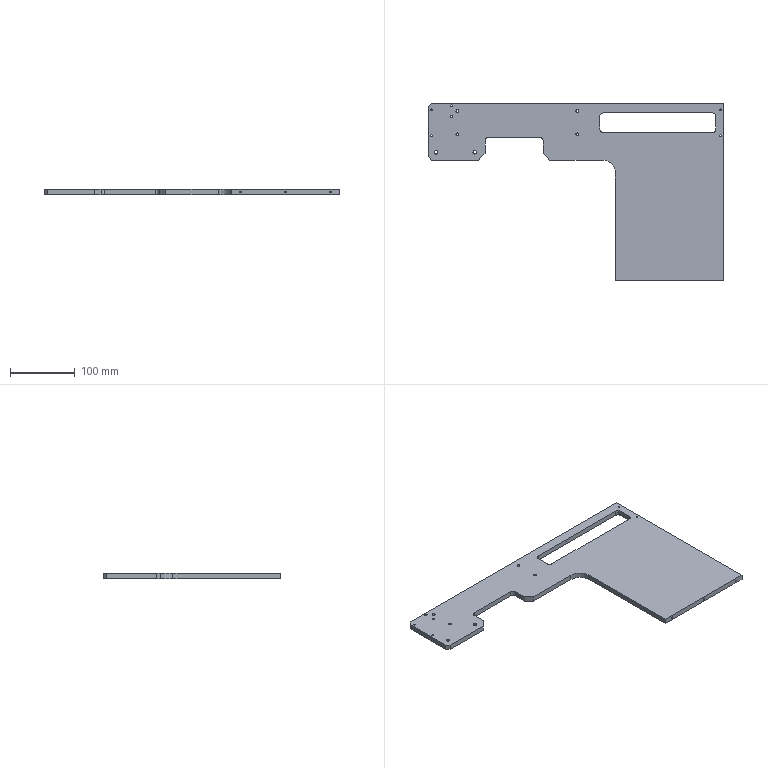Part | STEP file | CA-10-008Lift Stop Plate4_Default | 1 solid | 91 faces | box 458 x 275 x 8 mm | volume 503075 mm3 | cylinder 53 | plane 22 | cone 16 | commonest cylinder face diameters 2.5 x26 4.2 x8 10 x6 3.3 x4 5.5 x4 9.5 x4